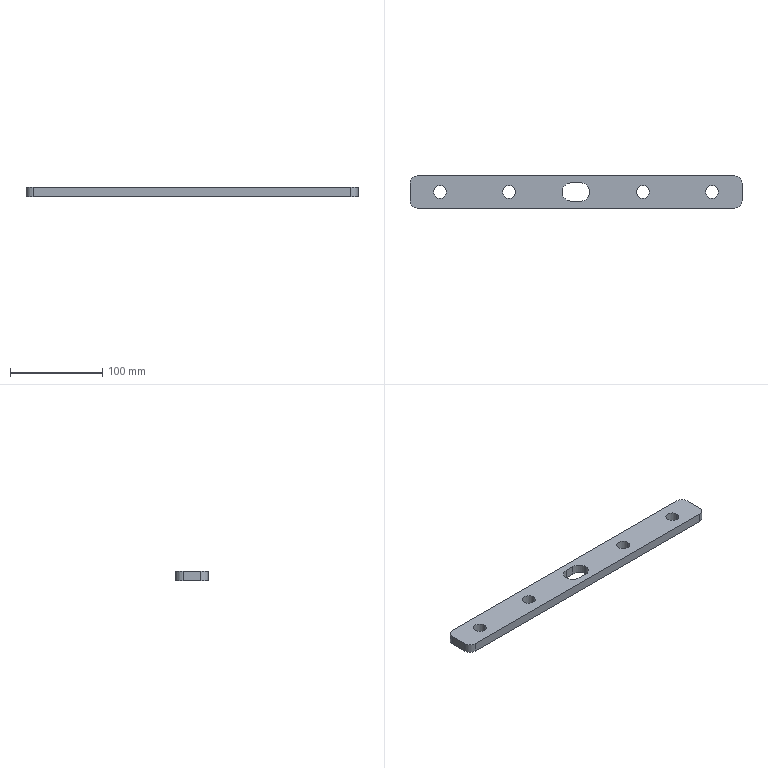Part | 1 solid | 23 faces | box 360 x 35 x 10 mm | volume 114152 mm3 | cylinder 15 | plane 8 | commonest cylinder face diameters 14 x8 16 x4 20 x3
STEP:
#1=CARTESIAN_POINT('',(79.5,0.,10.));
#2=VERTEX_POINT('',#1);
#3=CARTESIAN_POINT('',(65.5,0.,10.));
#4=VERTEX_POINT('',#3);
#5=CARTESIAN_POINT('',(72.5,0.,10.));
#6=DIRECTION('',(0.,0.,1.));
#7=DIRECTION('',(-1.,0.,0.));
#8=AXIS2_PLACEMENT_3D('',#5,#6,#7);
#9=CIRCLE('',#8,7.);
#10=EDGE_CURVE('',#2,#4,#9,.T.);
#11=ORIENTED_EDGE('',*,*,#10,.T.);
#12=CARTESIAN_POINT('',(65.5,0.,0.));
#13=VERTEX_POINT('',#12);
#14=CARTESIAN_POINT('',(65.5,0.,10.));
#15=DIRECTION('',(0.,0.,-1.));
#16=VECTOR('',#15,1000.);
#17=LINE('',#14,#16);
#18=EDGE_CURVE('',#4,#13,#17,.T.);
#19=ORIENTED_EDGE('',*,*,#18,.T.);
#20=CARTESIAN_POINT('',(79.5,0.,0.));
#21=VERTEX_POINT('',#20);
#22=CARTESIAN_POINT('',(72.5,0.,0.));
#23=DIRECTION('',(0.,0.,1.));
#24=DIRECTION('',(-1.,0.,0.));
#25=AXIS2_PLACEMENT_3D('',#22,#23,#24);
#26=CIRCLE('',#25,7.);
#27=EDGE_CURVE('',#21,#13,#26,.T.);
#28=ORIENTED_EDGE('',*,*,#27,.F.);
#29=CARTESIAN_POINT('',(79.5,0.,10.));
#30=DIRECTION('',(0.,0.,-1.));
#31=VECTOR('',#30,1000.);
#32=LINE('',#29,#31);
#33=EDGE_CURVE('',#2,#21,#32,.T.);
#34=ORIENTED_EDGE('',*,*,#33,.F.);
#35=EDGE_LOOP('',(#11,#19,#28,#34));
#36=FACE_OUTER_BOUND('',#35,.T.);
#37=CARTESIAN_POINT('',(72.5,0.,10.));
#38=DIRECTION('',(0.,0.,-1.));
#39=DIRECTION('',(1.,0.,0.));
#40=AXIS2_PLACEMENT_3D('',#37,#38,#39);
#41=CYLINDRICAL_SURFACE('',#40,7.);
#42=ADVANCED_FACE('',(#36),#41,.F.);
#43=CARTESIAN_POINT('',(154.5,0.,10.));
#44=VERTEX_POINT('',#43);
#45=CARTESIAN_POINT('',(140.5,0.,10.));
#46=VERTEX_POINT('',#45);
#47=CARTESIAN_POINT('',(147.5,0.,10.));
#48=DIRECTION('',(0.,0.,1.));
#49=DIRECTION('',(-1.,0.,0.));
#50=AXIS2_PLACEMENT_3D('',#47,#48,#49);
#51=CIRCLE('',#50,7.);
#52=EDGE_CURVE('',#44,#46,#51,.T.);
#53=ORIENTED_EDGE('',*,*,#52,.T.);
#54=CARTESIAN_POINT('',(140.5,0.,0.));
#55=VERTEX_POINT('',#54);
#56=CARTESIAN_POINT('',(140.5,0.,10.));
#57=DIRECTION('',(0.,0.,-1.));
#58=VECTOR('',#57,1000.);
#59=LINE('',#56,#58);
#60=EDGE_CURVE('',#46,#55,#59,.T.);
#61=ORIENTED_EDGE('',*,*,#60,.T.);
#62=CARTESIAN_POINT('',(154.5,0.,0.));
#63=VERTEX_POINT('',#62);
#64=CARTESIAN_POINT('',(147.5,0.,0.));
#65=DIRECTION('',(0.,0.,1.));
#66=DIRECTION('',(-1.,0.,0.));
#67=AXIS2_PLACEMENT_3D('',#64,#65,#66);
#68=CIRCLE('',#67,7.);
#69=EDGE_CURVE('',#63,#55,#68,.T.);
#70=ORIENTED_EDGE('',*,*,#69,.F.);
#71=CARTESIAN_POINT('',(154.5,0.,10.));
#72=DIRECTION('',(0.,0.,-1.));
#73=VECTOR('',#72,1000.);
#74=LINE('',#71,#73);
#75=EDGE_CURVE('',#44,#63,#74,.T.);
#76=ORIENTED_EDGE('',*,*,#75,.F.);
#77=EDGE_LOOP('',(#53,#61,#70,#76));
#78=FACE_OUTER_BOUND('',#77,.T.);
#79=CARTESIAN_POINT('',(147.5,0.,10.));
#80=DIRECTION('',(0.,0.,-1.));
#81=DIRECTION('',(1.,0.,0.));
#82=AXIS2_PLACEMENT_3D('',#79,#80,#81);
#83=CYLINDRICAL_SURFACE('',#82,7.);
#84=ADVANCED_FACE('',(#78),#83,.F.);
#85=CARTESIAN_POINT('',(-140.5,0.,10.));
#86=VERTEX_POINT('',#85);
#87=CARTESIAN_POINT('',(-154.5,0.,10.));
#88=VERTEX_POINT('',#87);
#89=CARTESIAN_POINT('',(-147.5,0.,10.));
#90=DIRECTION('',(0.,0.,1.));
#91=DIRECTION('',(1.,0.,0.));
#92=AXIS2_PLACEMENT_3D('',#89,#90,#91);
#93=CIRCLE('',#92,7.);
#94=EDGE_CURVE('',#86,#88,#93,.T.);
#95=ORIENTED_EDGE('',*,*,#94,.T.);
#96=CARTESIAN_POINT('',(-154.5,0.,0.));
#97=VERTEX_POINT('',#96);
#98=CARTESIAN_POINT('',(-154.5,0.,10.));
#99=DIRECTION('',(0.,0.,-1.));
#100=VECTOR('',#99,1000.);
#101=LINE('',#98,#100);
#102=EDGE_CURVE('',#88,#97,#101,.T.);
#103=ORIENTED_EDGE('',*,*,#102,.T.);
#104=CARTESIAN_POINT('',(-140.5,0.,0.));
#105=VERTEX_POINT('',#104);
#106=CARTESIAN_POINT('',(-147.5,0.,0.));
#107=DIRECTION('',(0.,0.,1.));
#108=DIRECTION('',(1.,0.,0.));
#109=AXIS2_PLACEMENT_3D('',#106,#107,#108);
#110=CIRCLE('',#109,7.);
#111=EDGE_CURVE('',#105,#97,#110,.T.);
#112=ORIENTED_EDGE('',*,*,#111,.F.);
#113=CARTESIAN_POINT('',(-140.5,0.,10.));
#114=DIRECTION('',(0.,0.,-1.));
#115=VECTOR('',#114,1000.);
#116=LINE('',#113,#115);
#117=EDGE_CURVE('',#86,#105,#116,.T.);
#118=ORIENTED_EDGE('',*,*,#117,.F.);
#119=EDGE_LOOP('',(#95,#103,#112,#118));
#120=FACE_OUTER_BOUND('',#119,.T.);
#121=CARTESIAN_POINT('',(-147.5,0.,10.));
#122=DIRECTION('',(0.,0.,-1.));
#123=DIRECTION('',(1.,0.,0.));
#124=AXIS2_PLACEMENT_3D('',#121,#122,#123);
#125=CYLINDRICAL_SURFACE('',#124,7.);
#126=ADVANCED_FACE('',(#120),#125,.F.);
#127=CARTESIAN_POINT('',(-65.5,0.,10.));
#128=VERTEX_POINT('',#127);
#129=CARTESIAN_POINT('',(-79.5,0.,10.));
#130=VERTEX_POINT('',#129);
#131=CARTESIAN_POINT('',(-72.5,0.,10.));
#132=DIRECTION('',(0.,0.,1.));
#133=DIRECTION('',(1.,0.,0.));
#134=AXIS2_PLACEMENT_3D('',#131,#132,#133);
#135=CIRCLE('',#134,7.);
#136=EDGE_CURVE('',#128,#130,#135,.T.);
#137=ORIENTED_EDGE('',*,*,#136,.T.);
#138=CARTESIAN_POINT('',(-79.5,0.,0.));
#139=VERTEX_POINT('',#138);
#140=CARTESIAN_POINT('',(-79.5,0.,10.));
#141=DIRECTION('',(0.,0.,-1.));
#142=VECTOR('',#141,1000.);
#143=LINE('',#140,#142);
#144=EDGE_CURVE('',#130,#139,#143,.T.);
#145=ORIENTED_EDGE('',*,*,#144,.T.);
#146=CARTESIAN_POINT('',(-65.5,0.,0.));
#147=VERTEX_POINT('',#146);
#148=CARTESIAN_POINT('',(-72.5,0.,0.));
#149=DIRECTION('',(0.,0.,1.));
#150=DIRECTION('',(1.,0.,0.));
#151=AXIS2_PLACEMENT_3D('',#148,#149,#150);
#152=CIRCLE('',#151,7.);
#153=EDGE_CURVE('',#147,#139,#152,.T.);
#154=ORIENTED_EDGE('',*,*,#153,.F.);
#155=CARTESIAN_POINT('',(-65.5,0.,10.));
#156=DIRECTION('',(0.,0.,-1.));
#157=VECTOR('',#156,1000.);
#158=LINE('',#155,#157);
#159=EDGE_CURVE('',#128,#147,#158,.T.);
#160=ORIENTED_EDGE('',*,*,#159,.F.);
#161=EDGE_LOOP('',(#137,#145,#154,#160));
#162=FACE_OUTER_BOUND('',#161,.T.);
#163=CARTESIAN_POINT('',(-72.5,0.,10.));
#164=DIRECTION('',(0.,0.,-1.));
#165=DIRECTION('',(1.,0.,0.));
#166=AXIS2_PLACEMENT_3D('',#163,#164,#165);
#167=CYLINDRICAL_SURFACE('',#166,7.);
#168=ADVANCED_FACE('',(#162),#167,.F.);
#169=CARTESIAN_POINT('',(5.,-10.,10.));
#170=VERTEX_POINT('',#169);
#171=CARTESIAN_POINT('',(15.,0.,10.));
#172=VERTEX_POINT('',#171);
#173=CARTESIAN_POINT('',(5.,0.,10.));
#174=DIRECTION('',(0.,0.,1.));
#175=DIRECTION('',(1.,0.,0.));
#176=AXIS2_PLACEMENT_3D('',#173,#174,#175);
#177=CIRCLE('',#176,10.);
#178=EDGE_CURVE('',#170,#172,#177,.T.);
#179=ORIENTED_EDGE('',*,*,#178,.T.);
#180=CARTESIAN_POINT('',(15.,0.,0.));
#181=VERTEX_POINT('',#180);
#182=CARTESIAN_POINT('',(15.,0.,10.));
#183=DIRECTION('',(0.,0.,-1.));
#184=VECTOR('',#183,1000.);
#185=LINE('',#182,#184);
#186=EDGE_CURVE('',#172,#181,#185,.T.);
#187=ORIENTED_EDGE('',*,*,#186,.T.);
#188=CARTESIAN_POINT('',(5.,-10.,0.));
#189=VERTEX_POINT('',#188);
#190=CARTESIAN_POINT('',(5.,0.,0.));
#191=DIRECTION('',(0.,0.,1.));
#192=DIRECTION('',(1.,0.,0.));
#193=AXIS2_PLACEMENT_3D('',#190,#191,#192);
#194=CIRCLE('',#193,10.);
#195=EDGE_CURVE('',#189,#181,#194,.T.);
#196=ORIENTED_EDGE('',*,*,#195,.F.);
#197=CARTESIAN_POINT('',(5.,-10.,10.));
#198=DIRECTION('',(0.,0.,-1.));
#199=VECTOR('',#198,1000.);
#200=LINE('',#197,#199);
#201=EDGE_CURVE('',#170,#189,#200,.T.);
#202=ORIENTED_EDGE('',*,*,#201,.F.);
#203=EDGE_LOOP('',(#179,#187,#196,#202));
#204=FACE_OUTER_BOUND('',#203,.T.);
#205=CARTESIAN_POINT('',(5.,0.,10.));
#206=DIRECTION('',(0.,0.,-1.));
#207=DIRECTION('',(1.,0.,0.));
#208=AXIS2_PLACEMENT_3D('',#205,#206,#207);
#209=CYLINDRICAL_SURFACE('',#208,10.);
#210=ADVANCED_FACE('',(#204),#209,.F.);
#211=CARTESIAN_POINT('',(180.,-9.5,0.));
#212=VERTEX_POINT('',#211);
#213=CARTESIAN_POINT('',(180.,9.5,0.));
#214=VERTEX_POINT('',#213);
#215=CARTESIAN_POINT('',(180.,17.5,0.));
#216=DIRECTION('',(0.,1.,0.));
#217=VECTOR('',#216,1000.);
#218=LINE('',#215,#217);
#219=EDGE_CURVE('',#212,#214,#218,.T.);
#220=ORIENTED_EDGE('',*,*,#219,.T.);
#221=CARTESIAN_POINT('',(180.,9.5,10.));
#222=VERTEX_POINT('',#221);
#223=CARTESIAN_POINT('',(180.,9.5,10.));
#224=DIRECTION('',(0.,0.,-1.));
#225=VECTOR('',#224,1000.);
#226=LINE('',#223,#225);
#227=EDGE_CURVE('',#222,#214,#226,.T.);
#228=ORIENTED_EDGE('',*,*,#227,.F.);
#229=CARTESIAN_POINT('',(180.,-9.5,10.));
#230=VERTEX_POINT('',#229);
#231=CARTESIAN_POINT('',(180.,17.5,10.));
#232=DIRECTION('',(0.,1.,0.));
#233=VECTOR('',#232,1000.);
#234=LINE('',#231,#233);
#235=EDGE_CURVE('',#230,#222,#234,.T.);
#236=ORIENTED_EDGE('',*,*,#235,.F.);
#237=CARTESIAN_POINT('',(180.,-9.5,10.));
#238=DIRECTION('',(0.,0.,1.));
#239=VECTOR('',#238,1000.);
#240=LINE('',#237,#239);
#241=EDGE_CURVE('',#212,#230,#240,.T.);
#242=ORIENTED_EDGE('',*,*,#241,.F.);
#243=EDGE_LOOP('',(#220,#228,#236,#242));
#244=FACE_OUTER_BOUND('',#243,.T.);
#245=CARTESIAN_POINT('',(180.,17.5,10.));
#246=DIRECTION('',(1.,0.,0.));
#247=DIRECTION('',(0.,0.,1.));
#248=AXIS2_PLACEMENT_3D('',#245,#246,#247);
#249=PLANE('',#248);
#250=ADVANCED_FACE('',(#244),#249,.T.);
#251=CARTESIAN_POINT('',(-172.,-17.5,10.));
#252=VERTEX_POINT('',#251);
#253=CARTESIAN_POINT('',(172.,-17.5,10.));
#254=VERTEX_POINT('',#253);
#255=CARTESIAN_POINT('',(-180.,-17.5,10.));
#256=DIRECTION('',(1.,0.,0.));
#257=VECTOR('',#256,1000.);
#258=LINE('',#255,#257);
#259=EDGE_CURVE('',#252,#254,#258,.T.);
#260=ORIENTED_EDGE('',*,*,#259,.F.);
#261=CARTESIAN_POINT('',(-172.,-17.5,0.));
#262=VERTEX_POINT('',#261);
#263=CARTESIAN_POINT('',(-172.,-17.5,10.));
#264=DIRECTION('',(0.,0.,1.));
#265=VECTOR('',#264,1000.);
#266=LINE('',#263,#265);
#267=EDGE_CURVE('',#262,#252,#266,.T.);
#268=ORIENTED_EDGE('',*,*,#267,.F.);
#269=CARTESIAN_POINT('',(172.,-17.5,0.));
#270=VERTEX_POINT('',#269);
#271=CARTESIAN_POINT('',(-180.,-17.5,0.));
#272=DIRECTION('',(1.,0.,0.));
#273=VECTOR('',#272,1000.);
#274=LINE('',#271,#273);
#275=EDGE_CURVE('',#262,#270,#274,.T.);
#276=ORIENTED_EDGE('',*,*,#275,.T.);
#277=CARTESIAN_POINT('',(172.,-17.5,10.));
#278=DIRECTION('',(0.,0.,-1.));
#279=VECTOR('',#278,1000.);
#280=LINE('',#277,#279);
#281=EDGE_CURVE('',#254,#270,#280,.T.);
#282=ORIENTED_EDGE('',*,*,#281,.F.);
#283=EDGE_LOOP('',(#260,#268,#276,#282));
#284=FACE_OUTER_BOUND('',#283,.T.);
#285=CARTESIAN_POINT('',(-180.,-17.5,10.));
#286=DIRECTION('',(0.,-1.,0.));
#287=DIRECTION('',(0.,0.,1.));
#288=AXIS2_PLACEMENT_3D('',#285,#286,#287);
#289=PLANE('',#288);
#290=ADVANCED_FACE('',(#284),#289,.T.);
#291=CARTESIAN_POINT('',(-180.,9.5,10.));
#292=VERTEX_POINT('',#291);
#293=CARTESIAN_POINT('',(-180.,-9.5,10.));
#294=VERTEX_POINT('',#293);
#295=CARTESIAN_POINT('',(-180.,17.5,10.));
#296=DIRECTION('',(0.,-1.,0.));
#297=VECTOR('',#296,1000.);
#298=LINE('',#295,#297);
#299=EDGE_CURVE('',#292,#294,#298,.T.);
#300=ORIENTED_EDGE('',*,*,#299,.F.);
#301=CARTESIAN_POINT('',(-180.,9.5,0.));
#302=VERTEX_POINT('',#301);
#303=CARTESIAN_POINT('',(-180.,9.5,10.));
#304=DIRECTION('',(0.,0.,1.));
#305=VECTOR('',#304,1000.);
#306=LINE('',#303,#305);
#307=EDGE_CURVE('',#302,#292,#306,.T.);
#308=ORIENTED_EDGE('',*,*,#307,.F.);
#309=CARTESIAN_POINT('',(-180.,-9.5,0.));
#310=VERTEX_POINT('',#309);
#311=CARTESIAN_POINT('',(-180.,17.5,0.));
#312=DIRECTION('',(0.,-1.,0.));
#313=VECTOR('',#312,1000.);
#314=LINE('',#311,#313);
#315=EDGE_CURVE('',#302,#310,#314,.T.);
#316=ORIENTED_EDGE('',*,*,#315,.T.);
#317=CARTESIAN_POINT('',(-180.,-9.5,10.));
#318=DIRECTION('',(0.,0.,-1.));
#319=VECTOR('',#318,1000.);
#320=LINE('',#317,#319);
#321=EDGE_CURVE('',#294,#310,#320,.T.);
#322=ORIENTED_EDGE('',*,*,#321,.F.);
#323=EDGE_LOOP('',(#300,#308,#316,#322));
#324=FACE_OUTER_BOUND('',#323,.T.);
#325=CARTESIAN_POINT('',(-180.,17.5,10.));
#326=DIRECTION('',(-1.,0.,0.));
#327=DIRECTION('',(0.,0.,-1.));
#328=AXIS2_PLACEMENT_3D('',#325,#326,#327);
#329=PLANE('',#328);
#330=ADVANCED_FACE('',(#324),#329,.T.);
#331=CARTESIAN_POINT('',(172.,17.5,0.));
#332=VERTEX_POINT('',#331);
#333=CARTESIAN_POINT('',(-172.,17.5,0.));
#334=VERTEX_POINT('',#333);
#335=CARTESIAN_POINT('',(-180.,17.5,0.));
#336=DIRECTION('',(-1.,0.,0.));
#337=VECTOR('',#336,1000.);
#338=LINE('',#335,#337);
#339=EDGE_CURVE('',#332,#334,#338,.T.);
#340=ORIENTED_EDGE('',*,*,#339,.T.);
#341=CARTESIAN_POINT('',(-172.,17.5,10.));
#342=VERTEX_POINT('',#341);
#343=CARTESIAN_POINT('',(-172.,17.5,10.));
#344=DIRECTION('',(0.,0.,-1.));
#345=VECTOR('',#344,1000.);
#346=LINE('',#343,#345);
#347=EDGE_CURVE('',#342,#334,#346,.T.);
#348=ORIENTED_EDGE('',*,*,#347,.F.);
#349=CARTESIAN_POINT('',(172.,17.5,10.));
#350=VERTEX_POINT('',#349);
#351=CARTESIAN_POINT('',(-180.,17.5,10.));
#352=DIRECTION('',(-1.,0.,0.));
#353=VECTOR('',#352,1000.);
#354=LINE('',#351,#353);
#355=EDGE_CURVE('',#350,#342,#354,.T.);
#356=ORIENTED_EDGE('',*,*,#355,.F.);
#357=CARTESIAN_POINT('',(172.,17.5,10.));
#358=DIRECTION('',(0.,0.,1.));
#359=VECTOR('',#358,1000.);
#360=LINE('',#357,#359);
#361=EDGE_CURVE('',#332,#350,#360,.T.);
#362=ORIENTED_EDGE('',*,*,#361,.F.);
#363=EDGE_LOOP('',(#340,#348,#356,#362));
#364=FACE_OUTER_BOUND('',#363,.T.);
#365=CARTESIAN_POINT('',(-180.,17.5,10.));
#366=DIRECTION('',(0.,1.,0.));
#367=DIRECTION('',(0.,0.,-1.));
#368=AXIS2_PLACEMENT_3D('',#365,#366,#367);
#369=PLANE('',#368);
#370=ADVANCED_FACE('',(#364),#369,.T.);
#371=ORIENTED_EDGE('',*,*,#10,.F.);
#372=CARTESIAN_POINT('',(72.5,0.,10.));
#373=DIRECTION('',(0.,0.,1.));
#374=DIRECTION('',(-1.,0.,0.));
#375=AXIS2_PLACEMENT_3D('',#372,#373,#374);
#376=CIRCLE('',#375,7.);
#377=EDGE_CURVE('',#4,#2,#376,.T.);
#378=ORIENTED_EDGE('',*,*,#377,.F.);
#379=EDGE_LOOP('',(#371,#378));
#380=FACE_BOUND('',#379,.T.);
#381=ORIENTED_EDGE('',*,*,#52,.F.);
#382=CARTESIAN_POINT('',(147.5,0.,10.));
#383=DIRECTION('',(0.,0.,1.));
#384=DIRECTION('',(-1.,0.,0.));
#385=AXIS2_PLACEMENT_3D('',#382,#383,#384);
#386=CIRCLE('',#385,7.);
#387=EDGE_CURVE('',#46,#44,#386,.T.);
#388=ORIENTED_EDGE('',*,*,#387,.F.);
#389=EDGE_LOOP('',(#381,#388));
#390=FACE_BOUND('',#389,.T.);
#391=ORIENTED_EDGE('',*,*,#94,.F.);
#392=CARTESIAN_POINT('',(-147.5,0.,10.));
#393=DIRECTION('',(0.,0.,1.));
#394=DIRECTION('',(1.,0.,0.));
#395=AXIS2_PLACEMENT_3D('',#392,#393,#394);
#396=CIRCLE('',#395,7.);
#397=EDGE_CURVE('',#88,#86,#396,.T.);
#398=ORIENTED_EDGE('',*,*,#397,.F.);
#399=EDGE_LOOP('',(#391,#398));
#400=FACE_BOUND('',#399,.T.);
#401=ORIENTED_EDGE('',*,*,#136,.F.);
#402=CARTESIAN_POINT('',(-72.5,0.,10.));
#403=DIRECTION('',(0.,0.,1.));
#404=DIRECTION('',(1.,0.,0.));
#405=AXIS2_PLACEMENT_3D('',#402,#403,#404);
#406=CIRCLE('',#405,7.);
#407=EDGE_CURVE('',#130,#128,#406,.T.);
#408=ORIENTED_EDGE('',*,*,#407,.F.);
#409=EDGE_LOOP('',(#401,#408));
#410=FACE_BOUND('',#409,.T.);
#411=CARTESIAN_POINT('',(5.,10.,10.));
#412=VERTEX_POINT('',#411);
#413=CARTESIAN_POINT('',(-5.,10.,10.));
#414=VERTEX_POINT('',#413);
#415=CARTESIAN_POINT('',(-5.,10.,10.));
#416=DIRECTION('',(-1.,0.,0.));
#417=VECTOR('',#416,1000.);
#418=LINE('',#415,#417);
#419=EDGE_CURVE('',#412,#414,#418,.T.);
#420=ORIENTED_EDGE('',*,*,#419,.F.);
#421=CARTESIAN_POINT('',(5.,0.,10.));
#422=DIRECTION('',(0.,0.,1.));
#423=DIRECTION('',(1.,0.,0.));
#424=AXIS2_PLACEMENT_3D('',#421,#422,#423);
#425=CIRCLE('',#424,10.);
#426=EDGE_CURVE('',#172,#412,#425,.T.);
#427=ORIENTED_EDGE('',*,*,#426,.F.);
#428=ORIENTED_EDGE('',*,*,#178,.F.);
#429=CARTESIAN_POINT('',(-5.,-10.,10.));
#430=VERTEX_POINT('',#429);
#431=CARTESIAN_POINT('',(-5.,-10.,10.));
#432=DIRECTION('',(1.,0.,0.));
#433=VECTOR('',#432,1000.);
#434=LINE('',#431,#433);
#435=EDGE_CURVE('',#430,#170,#434,.T.);
#436=ORIENTED_EDGE('',*,*,#435,.F.);
#437=CARTESIAN_POINT('',(-5.,0.,10.));
#438=DIRECTION('',(0.,0.,1.));
#439=DIRECTION('',(1.,0.,0.));
#440=AXIS2_PLACEMENT_3D('',#437,#438,#439);
#441=CIRCLE('',#440,10.);
#442=EDGE_CURVE('',#414,#430,#441,.T.);
#443=ORIENTED_EDGE('',*,*,#442,.F.);
#444=EDGE_LOOP('',(#420,#427,#428,#436,#443));
#445=FACE_BOUND('',#444,.T.);
#446=ORIENTED_EDGE('',*,*,#235,.T.);
#447=CARTESIAN_POINT('',(172.,9.5,10.));
#448=DIRECTION('',(0.,0.,-1.));
#449=DIRECTION('',(1.,0.,0.));
#450=AXIS2_PLACEMENT_3D('',#447,#448,#449);
#451=CIRCLE('',#450,8.);
#452=EDGE_CURVE('',#350,#222,#451,.T.);
#453=ORIENTED_EDGE('',*,*,#452,.F.);
#454=ORIENTED_EDGE('',*,*,#355,.T.);
#455=CARTESIAN_POINT('',(-172.,9.5,10.));
#456=DIRECTION('',(0.,0.,-1.));
#457=DIRECTION('',(1.,0.,0.));
#458=AXIS2_PLACEMENT_3D('',#455,#456,#457);
#459=CIRCLE('',#458,8.);
#460=EDGE_CURVE('',#292,#342,#459,.T.);
#461=ORIENTED_EDGE('',*,*,#460,.F.);
#462=ORIENTED_EDGE('',*,*,#299,.T.);
#463=CARTESIAN_POINT('',(-172.,-9.5,10.));
#464=DIRECTION('',(0.,0.,-1.));
#465=DIRECTION('',(1.,0.,0.));
#466=AXIS2_PLACEMENT_3D('',#463,#464,#465);
#467=CIRCLE('',#466,8.);
#468=EDGE_CURVE('',#252,#294,#467,.T.);
#469=ORIENTED_EDGE('',*,*,#468,.F.);
#470=ORIENTED_EDGE('',*,*,#259,.T.);
#471=CARTESIAN_POINT('',(172.,-9.5,10.));
#472=DIRECTION('',(0.,0.,-1.));
#473=DIRECTION('',(1.,0.,0.));
#474=AXIS2_PLACEMENT_3D('',#471,#472,#473);
#475=CIRCLE('',#474,8.);
#476=EDGE_CURVE('',#230,#254,#475,.T.);
#477=ORIENTED_EDGE('',*,*,#476,.F.);
#478=EDGE_LOOP('',(#446,#453,#454,#461,#462,#469,#470,#477));
#479=FACE_OUTER_BOUND('',#478,.T.);
#480=CARTESIAN_POINT('',(0.,0.,10.));
#481=DIRECTION('',(0.,0.,-1.));
#482=DIRECTION('',(1.,0.,0.));
#483=AXIS2_PLACEMENT_3D('',#480,#481,#482);
#484=PLANE('',#483);
#485=ADVANCED_FACE('',(#380,#390,#400,#410,#445,#479),#484,.F.);
#486=ORIENTED_EDGE('',*,*,#27,.T.);
#487=CARTESIAN_POINT('',(72.5,0.,0.));
#488=DIRECTION('',(0.,0.,1.));
#489=DIRECTION('',(-1.,0.,0.));
#490=AXIS2_PLACEMENT_3D('',#487,#488,#489);
#491=CIRCLE('',#490,7.);
#492=EDGE_CURVE('',#13,#21,#491,.T.);
#493=ORIENTED_EDGE('',*,*,#492,.T.);
#494=EDGE_LOOP('',(#486,#493));
#495=FACE_BOUND('',#494,.T.);
#496=ORIENTED_EDGE('',*,*,#69,.T.);
#497=CARTESIAN_POINT('',(147.5,0.,0.));
#498=DIRECTION('',(0.,0.,1.));
#499=DIRECTION('',(-1.,0.,0.));
#500=AXIS2_PLACEMENT_3D('',#497,#498,#499);
#501=CIRCLE('',#500,7.);
#502=EDGE_CURVE('',#55,#63,#501,.T.);
#503=ORIENTED_EDGE('',*,*,#502,.T.);
#504=EDGE_LOOP('',(#496,#503));
#505=FACE_BOUND('',#504,.T.);
#506=ORIENTED_EDGE('',*,*,#111,.T.);
#507=CARTESIAN_POINT('',(-147.5,0.,0.));
#508=DIRECTION('',(0.,0.,1.));
#509=DIRECTION('',(1.,0.,0.));
#510=AXIS2_PLACEMENT_3D('',#507,#508,#509);
#511=CIRCLE('',#510,7.);
#512=EDGE_CURVE('',#97,#105,#511,.T.);
#513=ORIENTED_EDGE('',*,*,#512,.T.);
#514=EDGE_LOOP('',(#506,#513));
#515=FACE_BOUND('',#514,.T.);
#516=ORIENTED_EDGE('',*,*,#153,.T.);
#517=CARTESIAN_POINT('',(-72.5,0.,0.));
#518=DIRECTION('',(0.,0.,1.));
#519=DIRECTION('',(1.,0.,0.));
#520=AXIS2_PLACEMENT_3D('',#517,#518,#519);
#521=CIRCLE('',#520,7.);
#522=EDGE_CURVE('',#139,#147,#521,.T.);
#523=ORIENTED_EDGE('',*,*,#522,.T.);
#524=EDGE_LOOP('',(#516,#523));
#525=FACE_BOUND('',#524,.T.);
#526=CARTESIAN_POINT('',(-5.,10.,0.));
#527=VERTEX_POINT('',#526);
#528=CARTESIAN_POINT('',(-5.,-10.,0.));
#529=VERTEX_POINT('',#528);
#530=CARTESIAN_POINT('',(-5.,0.,0.));
#531=DIRECTION('',(0.,0.,1.));
#532=DIRECTION('',(1.,0.,0.));
#533=AXIS2_PLACEMENT_3D('',#530,#531,#532);
#534=CIRCLE('',#533,10.);
#535=EDGE_CURVE('',#527,#529,#534,.T.);
#536=ORIENTED_EDGE('',*,*,#535,.T.);
#537=CARTESIAN_POINT('',(-5.,-10.,0.));
#538=DIRECTION('',(1.,0.,0.));
#539=VECTOR('',#538,1000.);
#540=LINE('',#537,#539);
#541=EDGE_CURVE('',#529,#189,#540,.T.);
#542=ORIENTED_EDGE('',*,*,#541,.T.);
#543=ORIENTED_EDGE('',*,*,#195,.T.);
#544=CARTESIAN_POINT('',(5.,10.,0.));
#545=VERTEX_POINT('',#544);
#546=CARTESIAN_POINT('',(5.,0.,0.));
#547=DIRECTION('',(0.,0.,1.));
#548=DIRECTION('',(1.,0.,0.));
#549=AXIS2_PLACEMENT_3D('',#546,#547,#548);
#550=CIRCLE('',#549,10.);
#551=EDGE_CURVE('',#181,#545,#550,.T.);
#552=ORIENTED_EDGE('',*,*,#551,.T.);
#553=CARTESIAN_POINT('',(-5.,10.,0.));
#554=DIRECTION('',(-1.,0.,0.));
#555=VECTOR('',#554,1000.);
#556=LINE('',#553,#555);
#557=EDGE_CURVE('',#545,#527,#556,.T.);
#558=ORIENTED_EDGE('',*,*,#557,.T.);
#559=EDGE_LOOP('',(#536,#542,#543,#552,#558));
#560=FACE_BOUND('',#559,.T.);
#561=ORIENTED_EDGE('',*,*,#275,.F.);
#562=CARTESIAN_POINT('',(-172.,-9.5,0.));
#563=DIRECTION('',(0.,0.,1.));
#564=DIRECTION('',(1.,0.,0.));
#565=AXIS2_PLACEMENT_3D('',#562,#563,#564);
#566=CIRCLE('',#565,8.);
#567=EDGE_CURVE('',#310,#262,#566,.T.);
#568=ORIENTED_EDGE('',*,*,#567,.F.);
#569=ORIENTED_EDGE('',*,*,#315,.F.);
#570=CARTESIAN_POINT('',(-172.,9.5,0.));
#571=DIRECTION('',(0.,0.,1.));
#572=DIRECTION('',(1.,0.,0.));
#573=AXIS2_PLACEMENT_3D('',#570,#571,#572);
#574=CIRCLE('',#573,8.);
#575=EDGE_CURVE('',#334,#302,#574,.T.);
#576=ORIENTED_EDGE('',*,*,#575,.F.);
#577=ORIENTED_EDGE('',*,*,#339,.F.);
#578=CARTESIAN_POINT('',(172.,9.5,0.));
#579=DIRECTION('',(0.,0.,1.));
#580=DIRECTION('',(1.,0.,0.));
#581=AXIS2_PLACEMENT_3D('',#578,#579,#580);
#582=CIRCLE('',#581,8.);
#583=EDGE_CURVE('',#214,#332,#582,.T.);
#584=ORIENTED_EDGE('',*,*,#583,.F.);
#585=ORIENTED_EDGE('',*,*,#219,.F.);
#586=CARTESIAN_POINT('',(172.,-9.5,0.));
#587=DIRECTION('',(0.,0.,1.));
#588=DIRECTION('',(1.,0.,0.));
#589=AXIS2_PLACEMENT_3D('',#586,#587,#588);
#590=CIRCLE('',#589,8.);
#591=EDGE_CURVE('',#270,#212,#590,.T.);
#592=ORIENTED_EDGE('',*,*,#591,.F.);
#593=EDGE_LOOP('',(#561,#568,#569,#576,#577,#584,#585,#592));
#594=FACE_OUTER_BOUND('',#593,.T.);
#595=CARTESIAN_POINT('',(0.,0.,0.));
#596=DIRECTION('',(0.,0.,-1.));
#597=DIRECTION('',(1.,0.,0.));
#598=AXIS2_PLACEMENT_3D('',#595,#596,#597);
#599=PLANE('',#598);
#600=ADVANCED_FACE('',(#495,#505,#515,#525,#560,#594),#599,.T.);
#601=ORIENTED_EDGE('',*,*,#535,.F.);
#602=CARTESIAN_POINT('',(-5.,10.,10.));
#603=DIRECTION('',(0.,0.,-1.));
#604=VECTOR('',#603,1000.);
#605=LINE('',#602,#604);
#606=EDGE_CURVE('',#414,#527,#605,.T.);
#607=ORIENTED_EDGE('',*,*,#606,.F.);
#608=ORIENTED_EDGE('',*,*,#442,.T.);
#609=CARTESIAN_POINT('',(-5.,-10.,10.));
#610=DIRECTION('',(0.,0.,-1.));
#611=VECTOR('',#610,1000.);
#612=LINE('',#609,#611);
#613=EDGE_CURVE('',#430,#529,#612,.T.);
#614=ORIENTED_EDGE('',*,*,#613,.T.);
#615=EDGE_LOOP('',(#601,#607,#608,#614));
#616=FACE_OUTER_BOUND('',#615,.T.);
#617=CARTESIAN_POINT('',(-5.,0.,10.));
#618=DIRECTION('',(0.,0.,-1.));
#619=DIRECTION('',(1.,0.,0.));
#620=AXIS2_PLACEMENT_3D('',#617,#618,#619);
#621=CYLINDRICAL_SURFACE('',#620,10.);
#622=ADVANCED_FACE('',(#616),#621,.F.);
#623=ORIENTED_EDGE('',*,*,#557,.F.);
#624=CARTESIAN_POINT('',(5.,10.,10.));
#625=DIRECTION('',(0.,0.,-1.));
#626=VECTOR('',#625,1000.);
#627=LINE('',#624,#626);
#628=EDGE_CURVE('',#412,#545,#627,.T.);
#629=ORIENTED_EDGE('',*,*,#628,.F.);
#630=ORIENTED_EDGE('',*,*,#419,.T.);
#631=ORIENTED_EDGE('',*,*,#606,.T.);
#632=EDGE_LOOP('',(#623,#629,#630,#631));
#633=FACE_OUTER_BOUND('',#632,.T.);
#634=CARTESIAN_POINT('',(-5.,10.,10.));
#635=DIRECTION('',(0.,1.,0.));
#636=DIRECTION('',(-1.,0.,0.));
#637=AXIS2_PLACEMENT_3D('',#634,#635,#636);
#638=PLANE('',#637);
#639=ADVANCED_FACE('',(#633),#638,.F.);
#640=ORIENTED_EDGE('',*,*,#186,.F.);
#641=ORIENTED_EDGE('',*,*,#426,.T.);
#642=ORIENTED_EDGE('',*,*,#628,.T.);
#643=ORIENTED_EDGE('',*,*,#551,.F.);
#644=EDGE_LOOP('',(#640,#641,#642,#643));
#645=FACE_OUTER_BOUND('',#644,.T.);
#646=CARTESIAN_POINT('',(5.,0.,10.));
#647=DIRECTION('',(0.,0.,-1.));
#648=DIRECTION('',(1.,0.,0.));
#649=AXIS2_PLACEMENT_3D('',#646,#647,#648);
#650=CYLINDRICAL_SURFACE('',#649,10.);
#651=ADVANCED_FACE('',(#645),#650,.F.);
#652=ORIENTED_EDGE('',*,*,#541,.F.);
#653=ORIENTED_EDGE('',*,*,#613,.F.);
#654=ORIENTED_EDGE('',*,*,#435,.T.);
#655=ORIENTED_EDGE('',*,*,#201,.T.);
#656=EDGE_LOOP('',(#652,#653,#654,#655));
#657=FACE_OUTER_BOUND('',#656,.T.);
#658=CARTESIAN_POINT('',(-5.,-10.,10.));
#659=DIRECTION('',(0.,-1.,0.));
#660=DIRECTION('',(0.,0.,1.));
#661=AXIS2_PLACEMENT_3D('',#658,#659,#660);
#662=PLANE('',#661);
#663=ADVANCED_FACE('',(#657),#662,.F.);
#664=ORIENTED_EDGE('',*,*,#144,.F.);
#665=ORIENTED_EDGE('',*,*,#407,.T.);
#666=ORIENTED_EDGE('',*,*,#159,.T.);
#667=ORIENTED_EDGE('',*,*,#522,.F.);
#668=EDGE_LOOP('',(#664,#665,#666,#667));
#669=FACE_OUTER_BOUND('',#668,.T.);
#670=CARTESIAN_POINT('',(-72.5,0.,10.));
#671=DIRECTION('',(0.,0.,-1.));
#672=DIRECTION('',(1.,0.,0.));
#673=AXIS2_PLACEMENT_3D('',#670,#671,#672);
#674=CYLINDRICAL_SURFACE('',#673,7.);
#675=ADVANCED_FACE('',(#669),#674,.F.);
#676=ORIENTED_EDGE('',*,*,#102,.F.);
#677=ORIENTED_EDGE('',*,*,#397,.T.);
#678=ORIENTED_EDGE('',*,*,#117,.T.);
#679=ORIENTED_EDGE('',*,*,#512,.F.);
#680=EDGE_LOOP('',(#676,#677,#678,#679));
#681=FACE_OUTER_BOUND('',#680,.T.);
#682=CARTESIAN_POINT('',(-147.5,0.,10.));
#683=DIRECTION('',(0.,0.,-1.));
#684=DIRECTION('',(1.,0.,0.));
#685=AXIS2_PLACEMENT_3D('',#682,#683,#684);
#686=CYLINDRICAL_SURFACE('',#685,7.);
#687=ADVANCED_FACE('',(#681),#686,.F.);
#688=ORIENTED_EDGE('',*,*,#60,.F.);
#689=ORIENTED_EDGE('',*,*,#387,.T.);
#690=ORIENTED_EDGE('',*,*,#75,.T.);
#691=ORIENTED_EDGE('',*,*,#502,.F.);
#692=EDGE_LOOP('',(#688,#689,#690,#691));
#693=FACE_OUTER_BOUND('',#692,.T.);
#694=CARTESIAN_POINT('',(147.5,0.,10.));
#695=DIRECTION('',(0.,0.,-1.));
#696=DIRECTION('',(1.,0.,0.));
#697=AXIS2_PLACEMENT_3D('',#694,#695,#696);
#698=CYLINDRICAL_SURFACE('',#697,7.);
#699=ADVANCED_FACE('',(#693),#698,.F.);
#700=ORIENTED_EDGE('',*,*,#18,.F.);
#701=ORIENTED_EDGE('',*,*,#377,.T.);
#702=ORIENTED_EDGE('',*,*,#33,.T.);
#703=ORIENTED_EDGE('',*,*,#492,.F.);
#704=EDGE_LOOP('',(#700,#701,#702,#703));
#705=FACE_OUTER_BOUND('',#704,.T.);
#706=CARTESIAN_POINT('',(72.5,0.,10.));
#707=DIRECTION('',(0.,0.,-1.));
#708=DIRECTION('',(1.,0.,0.));
#709=AXIS2_PLACEMENT_3D('',#706,#707,#708);
#710=CYLINDRICAL_SURFACE('',#709,7.);
#711=ADVANCED_FACE('',(#705),#710,.F.);
#712=ORIENTED_EDGE('',*,*,#476,.T.);
#713=ORIENTED_EDGE('',*,*,#281,.T.);
#714=ORIENTED_EDGE('',*,*,#591,.T.);
#715=ORIENTED_EDGE('',*,*,#241,.T.);
#716=EDGE_LOOP('',(#712,#713,#714,#715));
#717=FACE_OUTER_BOUND('',#716,.T.);
#718=CARTESIAN_POINT('',(172.,-9.5,10.));
#719=DIRECTION('',(0.,0.,-1.));
#720=DIRECTION('',(1.,0.,0.));
#721=AXIS2_PLACEMENT_3D('',#718,#719,#720);
#722=CYLINDRICAL_SURFACE('',#721,8.);
#723=ADVANCED_FACE('',(#717),#722,.T.);
#724=ORIENTED_EDGE('',*,*,#452,.T.);
#725=ORIENTED_EDGE('',*,*,#227,.T.);
#726=ORIENTED_EDGE('',*,*,#583,.T.);
#727=ORIENTED_EDGE('',*,*,#361,.T.);
#728=EDGE_LOOP('',(#724,#725,#726,#727));
#729=FACE_OUTER_BOUND('',#728,.T.);
#730=CARTESIAN_POINT('',(172.,9.5,10.));
#731=DIRECTION('',(0.,0.,-1.));
#732=DIRECTION('',(1.,0.,0.));
#733=AXIS2_PLACEMENT_3D('',#730,#731,#732);
#734=CYLINDRICAL_SURFACE('',#733,8.);
#735=ADVANCED_FACE('',(#729),#734,.T.);
#736=ORIENTED_EDGE('',*,*,#468,.T.);
#737=ORIENTED_EDGE('',*,*,#321,.T.);
#738=ORIENTED_EDGE('',*,*,#567,.T.);
#739=ORIENTED_EDGE('',*,*,#267,.T.);
#740=EDGE_LOOP('',(#736,#737,#738,#739));
#741=FACE_OUTER_BOUND('',#740,.T.);
#742=CARTESIAN_POINT('',(-172.,-9.5,10.));
#743=DIRECTION('',(0.,0.,-1.));
#744=DIRECTION('',(1.,0.,0.));
#745=AXIS2_PLACEMENT_3D('',#742,#743,#744);
#746=CYLINDRICAL_SURFACE('',#745,8.);
#747=ADVANCED_FACE('',(#741),#746,.T.);
#748=ORIENTED_EDGE('',*,*,#460,.T.);
#749=ORIENTED_EDGE('',*,*,#347,.T.);
#750=ORIENTED_EDGE('',*,*,#575,.T.);
#751=ORIENTED_EDGE('',*,*,#307,.T.);
#752=EDGE_LOOP('',(#748,#749,#750,#751));
#753=FACE_OUTER_BOUND('',#752,.T.);
#754=CARTESIAN_POINT('',(-172.,9.5,10.));
#755=DIRECTION('',(0.,0.,-1.));
#756=DIRECTION('',(1.,0.,0.));
#757=AXIS2_PLACEMENT_3D('',#754,#755,#756);
#758=CYLINDRICAL_SURFACE('',#757,8.);
#759=ADVANCED_FACE('',(#753),#758,.T.);
#760=CLOSED_SHELL('',(#42,#84,#126,#168,#210,#250,#290,#330,#370,#485,#600,#622,#639,#651,#663,#675,#687,#699,#711,#723,#735,#747,#759));
#761=MANIFOLD_SOLID_BREP('',#760);
#762=CARTESIAN_POINT('',(0.,0.,0.));
#763=DIRECTION('',(0.,0.,1.));
#764=DIRECTION('',(1.,0.,0.));
#765=AXIS2_PLACEMENT_3D('',#762,#763,#764);
#766=(LENGTH_UNIT()NAMED_UNIT(*)SI_UNIT(.MILLI.,.METRE.));
#767=UNCERTAINTY_MEASURE_WITH_UNIT(LENGTH_MEASURE(0.00001),#766,'','');
#768=(NAMED_UNIT(*)PLANE_ANGLE_UNIT()SI_UNIT($,.RADIAN.));
#769=(NAMED_UNIT(*)SI_UNIT($,.STERADIAN.)SOLID_ANGLE_UNIT());
#770=(GEOMETRIC_REPRESENTATION_CONTEXT(3)GLOBAL_UNCERTAINTY_ASSIGNED_CONTEXT((#767))GLOBAL_UNIT_ASSIGNED_CONTEXT((#766,#768,#769))REPRESENTATION_CONTEXT('',''));
#771=ADVANCED_BREP_SHAPE_REPRESENTATION('',(#761,#765),#770);